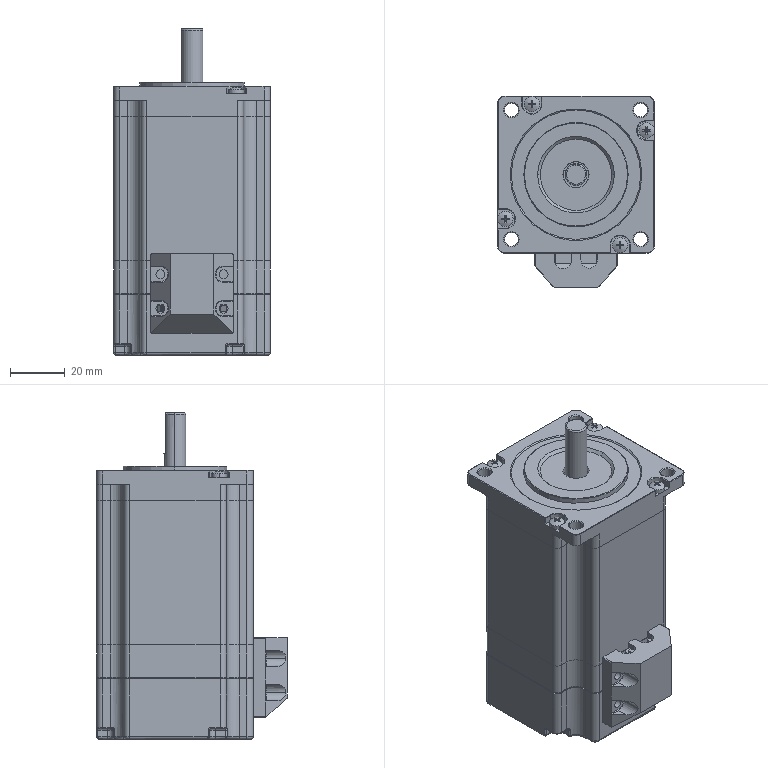Part | NX | features BREP 7 | 10 solids | 1966 faces | box 57.15 x 69.65 x 119 mm | volume 168268 mm3 | cone 1297 | cylinder 294 | plane 288 | torus 67 | spline 16 | sphere 4 | commonest cylinder face diameters 1 x57 4.6 x40 0.6 x31 3.2 x27 9.5 x20 2 x16